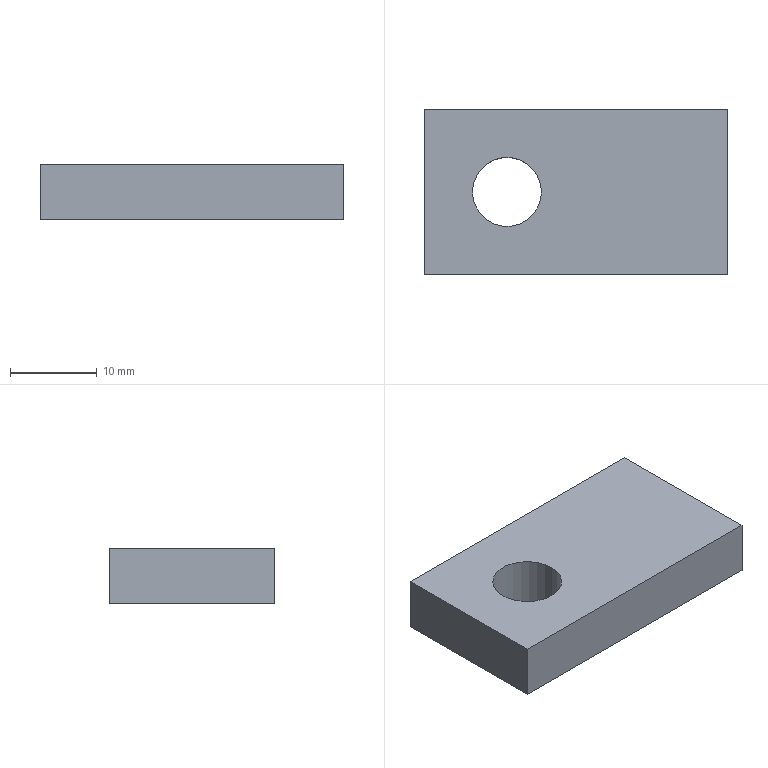Part | SolidWorks | features Extrusion 1 | 1 solid | 8 faces | box 34.925 x 19.05 x 6.35 mm | volume 3912 mm3 | plane 6 | cylinder 2 | commonest cylinder face diameters 7.925 x2
STEP:
#1=CARTESIAN_POINT('',(5.563,9.525,6.35));
#2=VERTEX_POINT('',#1);
#3=CARTESIAN_POINT('',(13.487,9.525,6.35));
#4=VERTEX_POINT('',#3);
#5=CARTESIAN_POINT('',(9.525,9.525,6.35));
#6=DIRECTION('',(0.,0.,1.));
#7=DIRECTION('',(1.,0.,0.));
#8=AXIS2_PLACEMENT_3D('',#5,#6,#7);
#9=CIRCLE('',#8,3.962);
#10=EDGE_CURVE('',#2,#4,#9,.T.);
#11=ORIENTED_EDGE('',*,*,#10,.T.);
#12=CARTESIAN_POINT('',(13.487,9.525,0.));
#13=VERTEX_POINT('',#12);
#14=CARTESIAN_POINT('',(13.487,9.525,6.35));
#15=DIRECTION('',(0.,0.,-1.));
#16=VECTOR('',#15,1000.);
#17=LINE('',#14,#16);
#18=EDGE_CURVE('',#4,#13,#17,.T.);
#19=ORIENTED_EDGE('',*,*,#18,.T.);
#20=CARTESIAN_POINT('',(5.563,9.525,0.));
#21=VERTEX_POINT('',#20);
#22=CARTESIAN_POINT('',(9.525,9.525,0.));
#23=DIRECTION('',(0.,0.,1.));
#24=DIRECTION('',(1.,0.,0.));
#25=AXIS2_PLACEMENT_3D('',#22,#23,#24);
#26=CIRCLE('',#25,3.962);
#27=EDGE_CURVE('',#21,#13,#26,.T.);
#28=ORIENTED_EDGE('',*,*,#27,.F.);
#29=CARTESIAN_POINT('',(5.563,9.525,6.35));
#30=DIRECTION('',(0.,0.,-1.));
#31=VECTOR('',#30,1000.);
#32=LINE('',#29,#31);
#33=EDGE_CURVE('',#2,#21,#32,.T.);
#34=ORIENTED_EDGE('',*,*,#33,.F.);
#35=EDGE_LOOP('',(#11,#19,#28,#34));
#36=FACE_OUTER_BOUND('',#35,.T.);
#37=CARTESIAN_POINT('',(9.525,9.525,6.35));
#38=DIRECTION('',(0.,0.,-1.));
#39=DIRECTION('',(-1.,0.,0.));
#40=AXIS2_PLACEMENT_3D('',#37,#38,#39);
#41=CYLINDRICAL_SURFACE('',#40,3.962);
#42=ADVANCED_FACE('',(#36),#41,.F.);
#43=CARTESIAN_POINT('',(0.,19.05,6.35));
#44=VERTEX_POINT('',#43);
#45=CARTESIAN_POINT('',(0.,0.,6.35));
#46=VERTEX_POINT('',#45);
#47=CARTESIAN_POINT('',(0.,0.,6.35));
#48=DIRECTION('',(0.,-1.,0.));
#49=VECTOR('',#48,1000.);
#50=LINE('',#47,#49);
#51=EDGE_CURVE('',#44,#46,#50,.T.);
#52=ORIENTED_EDGE('',*,*,#51,.T.);
#53=CARTESIAN_POINT('',(34.925,0.,6.35));
#54=VERTEX_POINT('',#53);
#55=CARTESIAN_POINT('',(0.,0.,6.35));
#56=DIRECTION('',(1.,0.,0.));
#57=VECTOR('',#56,1000.);
#58=LINE('',#55,#57);
#59=EDGE_CURVE('',#46,#54,#58,.T.);
#60=ORIENTED_EDGE('',*,*,#59,.T.);
#61=CARTESIAN_POINT('',(34.925,19.05,6.35));
#62=VERTEX_POINT('',#61);
#63=CARTESIAN_POINT('',(34.925,0.,6.35));
#64=DIRECTION('',(0.,1.,0.));
#65=VECTOR('',#64,1000.);
#66=LINE('',#63,#65);
#67=EDGE_CURVE('',#54,#62,#66,.T.);
#68=ORIENTED_EDGE('',*,*,#67,.T.);
#69=CARTESIAN_POINT('',(0.,19.05,6.35));
#70=DIRECTION('',(-1.,0.,0.));
#71=VECTOR('',#70,1000.);
#72=LINE('',#69,#71);
#73=EDGE_CURVE('',#62,#44,#72,.T.);
#74=ORIENTED_EDGE('',*,*,#73,.T.);
#75=EDGE_LOOP('',(#52,#60,#68,#74));
#76=FACE_OUTER_BOUND('',#75,.T.);
#77=ORIENTED_EDGE('',*,*,#10,.F.);
#78=CARTESIAN_POINT('',(9.525,9.525,6.35));
#79=DIRECTION('',(0.,0.,1.));
#80=DIRECTION('',(1.,0.,0.));
#81=AXIS2_PLACEMENT_3D('',#78,#79,#80);
#82=CIRCLE('',#81,3.962);
#83=EDGE_CURVE('',#4,#2,#82,.T.);
#84=ORIENTED_EDGE('',*,*,#83,.F.);
#85=EDGE_LOOP('',(#77,#84));
#86=FACE_BOUND('',#85,.T.);
#87=CARTESIAN_POINT('',(0.,0.,6.35));
#88=DIRECTION('',(0.,0.,-1.));
#89=DIRECTION('',(-1.,0.,0.));
#90=AXIS2_PLACEMENT_3D('',#87,#88,#89);
#91=PLANE('',#90);
#92=ADVANCED_FACE('',(#76,#86),#91,.F.);
#93=CARTESIAN_POINT('',(0.,19.05,0.));
#94=VERTEX_POINT('',#93);
#95=CARTESIAN_POINT('',(0.,0.,0.));
#96=VERTEX_POINT('',#95);
#97=CARTESIAN_POINT('',(0.,0.,0.));
#98=DIRECTION('',(0.,-1.,0.));
#99=VECTOR('',#98,1000.);
#100=LINE('',#97,#99);
#101=EDGE_CURVE('',#94,#96,#100,.T.);
#102=ORIENTED_EDGE('',*,*,#101,.F.);
#103=CARTESIAN_POINT('',(34.925,19.05,0.));
#104=VERTEX_POINT('',#103);
#105=CARTESIAN_POINT('',(0.,19.05,0.));
#106=DIRECTION('',(-1.,0.,0.));
#107=VECTOR('',#106,1000.);
#108=LINE('',#105,#107);
#109=EDGE_CURVE('',#104,#94,#108,.T.);
#110=ORIENTED_EDGE('',*,*,#109,.F.);
#111=CARTESIAN_POINT('',(34.925,0.,0.));
#112=VERTEX_POINT('',#111);
#113=CARTESIAN_POINT('',(34.925,0.,0.));
#114=DIRECTION('',(0.,1.,0.));
#115=VECTOR('',#114,1000.);
#116=LINE('',#113,#115);
#117=EDGE_CURVE('',#112,#104,#116,.T.);
#118=ORIENTED_EDGE('',*,*,#117,.F.);
#119=CARTESIAN_POINT('',(0.,0.,0.));
#120=DIRECTION('',(1.,0.,0.));
#121=VECTOR('',#120,1000.);
#122=LINE('',#119,#121);
#123=EDGE_CURVE('',#96,#112,#122,.T.);
#124=ORIENTED_EDGE('',*,*,#123,.F.);
#125=EDGE_LOOP('',(#102,#110,#118,#124));
#126=FACE_OUTER_BOUND('',#125,.T.);
#127=ORIENTED_EDGE('',*,*,#27,.T.);
#128=CARTESIAN_POINT('',(9.525,9.525,0.));
#129=DIRECTION('',(0.,0.,1.));
#130=DIRECTION('',(1.,0.,0.));
#131=AXIS2_PLACEMENT_3D('',#128,#129,#130);
#132=CIRCLE('',#131,3.962);
#133=EDGE_CURVE('',#13,#21,#132,.T.);
#134=ORIENTED_EDGE('',*,*,#133,.T.);
#135=EDGE_LOOP('',(#127,#134));
#136=FACE_BOUND('',#135,.T.);
#137=CARTESIAN_POINT('',(0.,0.,0.));
#138=DIRECTION('',(0.,0.,-1.));
#139=DIRECTION('',(-1.,0.,0.));
#140=AXIS2_PLACEMENT_3D('',#137,#138,#139);
#141=PLANE('',#140);
#142=ADVANCED_FACE('',(#126,#136),#141,.T.);
#143=ORIENTED_EDGE('',*,*,#101,.T.);
#144=CARTESIAN_POINT('',(0.,0.,6.35));
#145=DIRECTION('',(0.,0.,-1.));
#146=VECTOR('',#145,1000.);
#147=LINE('',#144,#146);
#148=EDGE_CURVE('',#46,#96,#147,.T.);
#149=ORIENTED_EDGE('',*,*,#148,.F.);
#150=ORIENTED_EDGE('',*,*,#51,.F.);
#151=CARTESIAN_POINT('',(0.,19.05,6.35));
#152=DIRECTION('',(0.,0.,-1.));
#153=VECTOR('',#152,1000.);
#154=LINE('',#151,#153);
#155=EDGE_CURVE('',#44,#94,#154,.T.);
#156=ORIENTED_EDGE('',*,*,#155,.T.);
#157=EDGE_LOOP('',(#143,#149,#150,#156));
#158=FACE_OUTER_BOUND('',#157,.T.);
#159=CARTESIAN_POINT('',(0.,0.,6.35));
#160=DIRECTION('',(1.,0.,0.));
#161=DIRECTION('',(0.,0.,-1.));
#162=AXIS2_PLACEMENT_3D('',#159,#160,#161);
#163=PLANE('',#162);
#164=ADVANCED_FACE('',(#158),#163,.F.);
#165=ORIENTED_EDGE('',*,*,#123,.T.);
#166=CARTESIAN_POINT('',(34.925,0.,6.35));
#167=DIRECTION('',(0.,0.,-1.));
#168=VECTOR('',#167,1000.);
#169=LINE('',#166,#168);
#170=EDGE_CURVE('',#54,#112,#169,.T.);
#171=ORIENTED_EDGE('',*,*,#170,.F.);
#172=ORIENTED_EDGE('',*,*,#59,.F.);
#173=ORIENTED_EDGE('',*,*,#148,.T.);
#174=EDGE_LOOP('',(#165,#171,#172,#173));
#175=FACE_OUTER_BOUND('',#174,.T.);
#176=CARTESIAN_POINT('',(0.,0.,6.35));
#177=DIRECTION('',(0.,1.,0.));
#178=DIRECTION('',(0.,0.,1.));
#179=AXIS2_PLACEMENT_3D('',#176,#177,#178);
#180=PLANE('',#179);
#181=ADVANCED_FACE('',(#175),#180,.F.);
#182=ORIENTED_EDGE('',*,*,#117,.T.);
#183=CARTESIAN_POINT('',(34.925,19.05,6.35));
#184=DIRECTION('',(0.,0.,-1.));
#185=VECTOR('',#184,1000.);
#186=LINE('',#183,#185);
#187=EDGE_CURVE('',#62,#104,#186,.T.);
#188=ORIENTED_EDGE('',*,*,#187,.F.);
#189=ORIENTED_EDGE('',*,*,#67,.F.);
#190=ORIENTED_EDGE('',*,*,#170,.T.);
#191=EDGE_LOOP('',(#182,#188,#189,#190));
#192=FACE_OUTER_BOUND('',#191,.T.);
#193=CARTESIAN_POINT('',(34.925,0.,6.35));
#194=DIRECTION('',(-1.,0.,0.));
#195=DIRECTION('',(0.,0.,1.));
#196=AXIS2_PLACEMENT_3D('',#193,#194,#195);
#197=PLANE('',#196);
#198=ADVANCED_FACE('',(#192),#197,.F.);
#199=ORIENTED_EDGE('',*,*,#109,.T.);
#200=ORIENTED_EDGE('',*,*,#155,.F.);
#201=ORIENTED_EDGE('',*,*,#73,.F.);
#202=ORIENTED_EDGE('',*,*,#187,.T.);
#203=EDGE_LOOP('',(#199,#200,#201,#202));
#204=FACE_OUTER_BOUND('',#203,.T.);
#205=CARTESIAN_POINT('',(0.,19.05,6.35));
#206=DIRECTION('',(0.,-1.,0.));
#207=DIRECTION('',(0.,0.,-1.));
#208=AXIS2_PLACEMENT_3D('',#205,#206,#207);
#209=PLANE('',#208);
#210=ADVANCED_FACE('',(#204),#209,.F.);
#211=ORIENTED_EDGE('',*,*,#18,.F.);
#212=ORIENTED_EDGE('',*,*,#83,.T.);
#213=ORIENTED_EDGE('',*,*,#33,.T.);
#214=ORIENTED_EDGE('',*,*,#133,.F.);
#215=EDGE_LOOP('',(#211,#212,#213,#214));
#216=FACE_OUTER_BOUND('',#215,.T.);
#217=CARTESIAN_POINT('',(9.525,9.525,6.35));
#218=DIRECTION('',(0.,0.,-1.));
#219=DIRECTION('',(-1.,0.,0.));
#220=AXIS2_PLACEMENT_3D('',#217,#218,#219);
#221=CYLINDRICAL_SURFACE('',#220,3.962);
#222=ADVANCED_FACE('',(#216),#221,.F.);
#223=CLOSED_SHELL('',(#42,#92,#142,#164,#181,#198,#210,#222));
#224=MANIFOLD_SOLID_BREP('',#223);
#225=CARTESIAN_POINT('',(0.,0.,0.));
#226=DIRECTION('',(0.,0.,1.));
#227=DIRECTION('',(1.,0.,0.));
#228=AXIS2_PLACEMENT_3D('',#225,#226,#227);
#229=(LENGTH_UNIT()NAMED_UNIT(*)SI_UNIT(.MILLI.,.METRE.));
#230=UNCERTAINTY_MEASURE_WITH_UNIT(LENGTH_MEASURE(0.00001),#229,'','');
#231=(NAMED_UNIT(*)PLANE_ANGLE_UNIT()SI_UNIT($,.RADIAN.));
#232=(NAMED_UNIT(*)SI_UNIT($,.STERADIAN.)SOLID_ANGLE_UNIT());
#233=(GEOMETRIC_REPRESENTATION_CONTEXT(3)GLOBAL_UNCERTAINTY_ASSIGNED_CONTEXT((#230))GLOBAL_UNIT_ASSIGNED_CONTEXT((#229,#231,#232))REPRESENTATION_CONTEXT('',''));
#234=ADVANCED_BREP_SHAPE_REPRESENTATION('',(#224,#228),#233);